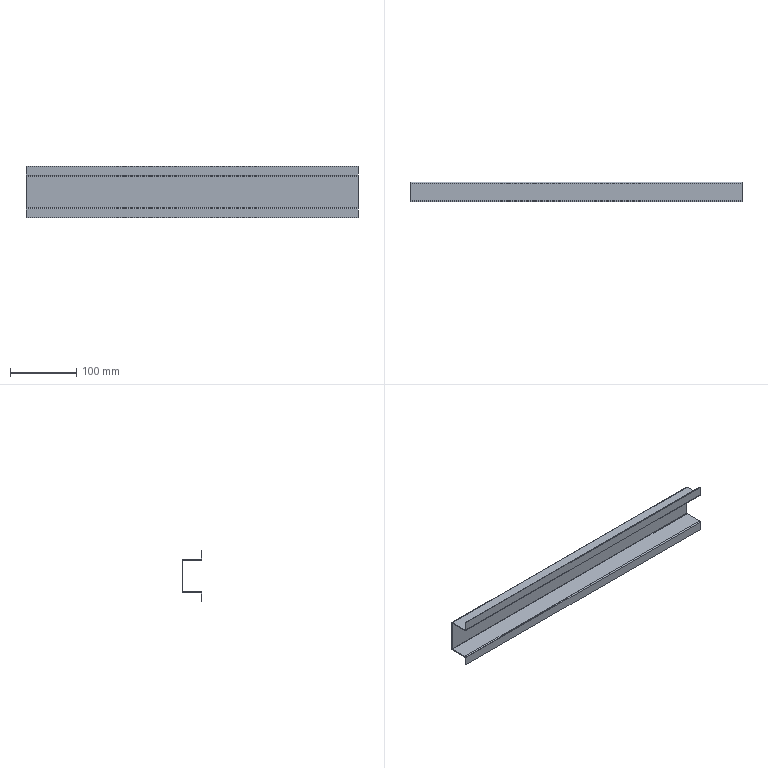Part | SolidWorks | features EdgeFlange 2, FlatPattern 1, SMBaseFlange 1, SheetMetal 1 | 1 solid | 38 faces | box 500 x 30 x 77.6 mm | volume 80038 mm3 | plane 30 | cylinder 8 | commonest cylinder face diameters 0.9 x4 3.3 x4
STEP:
#1=CARTESIAN_POINT('',(-250.,-0.45,-25.));
#2=VERTEX_POINT('',#1);
#3=CARTESIAN_POINT('',(-250.,-27.15,-25.));
#4=VERTEX_POINT('',#3);
#5=CARTESIAN_POINT('',(-250.,0.,-25.));
#6=DIRECTION('',(0.,-1.,0.));
#7=VECTOR('',#6,1000.);
#8=LINE('',#5,#7);
#9=EDGE_CURVE('',#2,#4,#8,.T.);
#10=ORIENTED_EDGE('',*,*,#9,.T.);
#11=CARTESIAN_POINT('',(-250.,-27.15,-23.8));
#12=VERTEX_POINT('',#11);
#13=CARTESIAN_POINT('',(-250.,-27.15,-25.));
#14=DIRECTION('',(0.,0.,1.));
#15=VECTOR('',#14,1000.);
#16=LINE('',#13,#15);
#17=EDGE_CURVE('',#4,#12,#16,.T.);
#18=ORIENTED_EDGE('',*,*,#17,.T.);
#19=CARTESIAN_POINT('',(-250.,-0.45,-23.8));
#20=VERTEX_POINT('',#19);
#21=CARTESIAN_POINT('',(-250.,-28.8,-23.8));
#22=DIRECTION('',(0.,-1.,0.));
#23=VECTOR('',#22,1000.);
#24=LINE('',#21,#23);
#25=EDGE_CURVE('',#20,#12,#24,.T.);
#26=ORIENTED_EDGE('',*,*,#25,.F.);
#27=CARTESIAN_POINT('',(-250.,-0.45,-25.));
#28=DIRECTION('',(0.,0.,-1.));
#29=VECTOR('',#28,1000.);
#30=LINE('',#27,#29);
#31=EDGE_CURVE('',#20,#2,#30,.T.);
#32=ORIENTED_EDGE('',*,*,#31,.T.);
#33=EDGE_LOOP('',(#10,#18,#26,#32));
#34=FACE_OUTER_BOUND('',#33,.T.);
#35=CARTESIAN_POINT('',(-250.,0.,-25.));
#36=DIRECTION('',(-1.,0.,0.));
#37=DIRECTION('',(0.,0.,1.));
#38=AXIS2_PLACEMENT_3D('',#35,#36,#37);
#39=PLANE('',#38);
#40=ADVANCED_FACE('',(#34),#39,.T.);
#41=CARTESIAN_POINT('',(250.,-27.15,-25.));
#42=VERTEX_POINT('',#41);
#43=CARTESIAN_POINT('',(-250.,-27.15,-25.));
#44=DIRECTION('',(1.,0.,0.));
#45=VECTOR('',#44,1000.);
#46=LINE('',#43,#45);
#47=EDGE_CURVE('',#4,#42,#46,.T.);
#48=ORIENTED_EDGE('',*,*,#47,.F.);
#49=ORIENTED_EDGE('',*,*,#9,.F.);
#50=CARTESIAN_POINT('',(250.,-0.45,-25.));
#51=VERTEX_POINT('',#50);
#52=CARTESIAN_POINT('',(-250.,-0.45,-25.));
#53=DIRECTION('',(-1.,0.,0.));
#54=VECTOR('',#53,1000.);
#55=LINE('',#52,#54);
#56=EDGE_CURVE('',#51,#2,#55,.T.);
#57=ORIENTED_EDGE('',*,*,#56,.F.);
#58=CARTESIAN_POINT('',(250.,-28.8,-25.));
#59=DIRECTION('',(0.,1.,0.));
#60=VECTOR('',#59,1000.);
#61=LINE('',#58,#60);
#62=EDGE_CURVE('',#42,#51,#61,.T.);
#63=ORIENTED_EDGE('',*,*,#62,.F.);
#64=EDGE_LOOP('',(#48,#49,#57,#63));
#65=FACE_OUTER_BOUND('',#64,.T.);
#66=CARTESIAN_POINT('',(-250.,-28.8,-25.));
#67=DIRECTION('',(0.,0.,1.));
#68=DIRECTION('',(0.,-1.,0.));
#69=AXIS2_PLACEMENT_3D('',#66,#67,#68);
#70=PLANE('',#69);
#71=ADVANCED_FACE('',(#65),#70,.F.);
#72=ORIENTED_EDGE('',*,*,#25,.T.);
#73=CARTESIAN_POINT('',(250.,-27.15,-23.8));
#74=VERTEX_POINT('',#73);
#75=CARTESIAN_POINT('',(-250.,-27.15,-23.8));
#76=DIRECTION('',(1.,0.,0.));
#77=VECTOR('',#76,1000.);
#78=LINE('',#75,#77);
#79=EDGE_CURVE('',#12,#74,#78,.T.);
#80=ORIENTED_EDGE('',*,*,#79,.T.);
#81=CARTESIAN_POINT('',(250.,-0.45,-23.8));
#82=VERTEX_POINT('',#81);
#83=CARTESIAN_POINT('',(250.,-28.8,-23.8));
#84=DIRECTION('',(0.,1.,0.));
#85=VECTOR('',#84,1000.);
#86=LINE('',#83,#85);
#87=EDGE_CURVE('',#74,#82,#86,.T.);
#88=ORIENTED_EDGE('',*,*,#87,.T.);
#89=CARTESIAN_POINT('',(-250.,-0.45,-23.8));
#90=DIRECTION('',(1.,0.,0.));
#91=VECTOR('',#90,1000.);
#92=LINE('',#89,#91);
#93=EDGE_CURVE('',#20,#82,#92,.T.);
#94=ORIENTED_EDGE('',*,*,#93,.F.);
#95=EDGE_LOOP('',(#72,#80,#88,#94));
#96=FACE_OUTER_BOUND('',#95,.T.);
#97=CARTESIAN_POINT('',(-250.,-28.8,-23.8));
#98=DIRECTION('',(0.,0.,1.));
#99=DIRECTION('',(0.,-1.,0.));
#100=AXIS2_PLACEMENT_3D('',#97,#98,#99);
#101=PLANE('',#100);
#102=ADVANCED_FACE('',(#96),#101,.T.);
#103=CARTESIAN_POINT('',(250.,-0.45,25.));
#104=VERTEX_POINT('',#103);
#105=CARTESIAN_POINT('',(250.,-27.15,25.));
#106=VERTEX_POINT('',#105);
#107=CARTESIAN_POINT('',(250.,-28.8,25.));
#108=DIRECTION('',(0.,-1.,0.));
#109=VECTOR('',#108,1000.);
#110=LINE('',#107,#109);
#111=EDGE_CURVE('',#104,#106,#110,.T.);
#112=ORIENTED_EDGE('',*,*,#111,.T.);
#113=CARTESIAN_POINT('',(250.,-27.15,23.8));
#114=VERTEX_POINT('',#113);
#115=CARTESIAN_POINT('',(250.,-27.15,25.));
#116=DIRECTION('',(0.,0.,-1.));
#117=VECTOR('',#116,1000.);
#118=LINE('',#115,#117);
#119=EDGE_CURVE('',#106,#114,#118,.T.);
#120=ORIENTED_EDGE('',*,*,#119,.T.);
#121=CARTESIAN_POINT('',(250.,-0.45,23.8));
#122=VERTEX_POINT('',#121);
#123=CARTESIAN_POINT('',(250.,0.,23.8));
#124=DIRECTION('',(0.,-1.,0.));
#125=VECTOR('',#124,1000.);
#126=LINE('',#123,#125);
#127=EDGE_CURVE('',#122,#114,#126,.T.);
#128=ORIENTED_EDGE('',*,*,#127,.F.);
#129=CARTESIAN_POINT('',(250.,-0.45,25.));
#130=DIRECTION('',(0.,0.,1.));
#131=VECTOR('',#130,1000.);
#132=LINE('',#129,#131);
#133=EDGE_CURVE('',#122,#104,#132,.T.);
#134=ORIENTED_EDGE('',*,*,#133,.T.);
#135=EDGE_LOOP('',(#112,#120,#128,#134));
#136=FACE_OUTER_BOUND('',#135,.T.);
#137=CARTESIAN_POINT('',(250.,-28.8,25.));
#138=DIRECTION('',(1.,0.,0.));
#139=DIRECTION('',(0.,0.,-1.));
#140=AXIS2_PLACEMENT_3D('',#137,#138,#139);
#141=PLANE('',#140);
#142=ADVANCED_FACE('',(#136),#141,.T.);
#143=CARTESIAN_POINT('',(-250.,-27.15,25.));
#144=VERTEX_POINT('',#143);
#145=CARTESIAN_POINT('',(-250.,-0.45,25.));
#146=VERTEX_POINT('',#145);
#147=CARTESIAN_POINT('',(-250.,0.,25.));
#148=DIRECTION('',(0.,1.,0.));
#149=VECTOR('',#148,1000.);
#150=LINE('',#147,#149);
#151=EDGE_CURVE('',#144,#146,#150,.T.);
#152=ORIENTED_EDGE('',*,*,#151,.F.);
#153=CARTESIAN_POINT('',(250.,-27.15,25.));
#154=DIRECTION('',(-1.,0.,0.));
#155=VECTOR('',#154,1000.);
#156=LINE('',#153,#155);
#157=EDGE_CURVE('',#106,#144,#156,.T.);
#158=ORIENTED_EDGE('',*,*,#157,.F.);
#159=ORIENTED_EDGE('',*,*,#111,.F.);
#160=CARTESIAN_POINT('',(-250.,-0.45,25.));
#161=DIRECTION('',(-1.,0.,0.));
#162=VECTOR('',#161,1000.);
#163=LINE('',#160,#162);
#164=EDGE_CURVE('',#104,#146,#163,.T.);
#165=ORIENTED_EDGE('',*,*,#164,.T.);
#166=EDGE_LOOP('',(#152,#158,#159,#165));
#167=FACE_OUTER_BOUND('',#166,.T.);
#168=CARTESIAN_POINT('',(-250.,0.,25.));
#169=DIRECTION('',(0.,0.,1.));
#170=DIRECTION('',(0.,-1.,0.));
#171=AXIS2_PLACEMENT_3D('',#168,#169,#170);
#172=PLANE('',#171);
#173=ADVANCED_FACE('',(#167),#172,.T.);
#174=CARTESIAN_POINT('',(-250.,-27.15,23.8));
#175=VERTEX_POINT('',#174);
#176=CARTESIAN_POINT('',(250.,-27.15,23.8));
#177=DIRECTION('',(-1.,0.,0.));
#178=VECTOR('',#177,1000.);
#179=LINE('',#176,#178);
#180=EDGE_CURVE('',#114,#175,#179,.T.);
#181=ORIENTED_EDGE('',*,*,#180,.T.);
#182=CARTESIAN_POINT('',(-250.,-0.45,23.8));
#183=VERTEX_POINT('',#182);
#184=CARTESIAN_POINT('',(-250.,0.,23.8));
#185=DIRECTION('',(0.,1.,0.));
#186=VECTOR('',#185,1000.);
#187=LINE('',#184,#186);
#188=EDGE_CURVE('',#175,#183,#187,.T.);
#189=ORIENTED_EDGE('',*,*,#188,.T.);
#190=CARTESIAN_POINT('',(250.,-0.45,23.8));
#191=DIRECTION('',(-1.,0.,0.));
#192=VECTOR('',#191,1000.);
#193=LINE('',#190,#192);
#194=EDGE_CURVE('',#122,#183,#193,.T.);
#195=ORIENTED_EDGE('',*,*,#194,.F.);
#196=ORIENTED_EDGE('',*,*,#127,.T.);
#197=EDGE_LOOP('',(#181,#189,#195,#196));
#198=FACE_OUTER_BOUND('',#197,.T.);
#199=CARTESIAN_POINT('',(-250.,0.,23.8));
#200=DIRECTION('',(0.,0.,1.));
#201=DIRECTION('',(0.,-1.,0.));
#202=AXIS2_PLACEMENT_3D('',#199,#200,#201);
#203=PLANE('',#202);
#204=ADVANCED_FACE('',(#198),#203,.F.);
#205=CARTESIAN_POINT('',(-250.,0.,-23.35));
#206=VERTEX_POINT('',#205);
#207=CARTESIAN_POINT('',(-250.,1.2,-23.35));
#208=VERTEX_POINT('',#207);
#209=CARTESIAN_POINT('',(-250.,0.,-23.35));
#210=DIRECTION('',(0.,1.,0.));
#211=VECTOR('',#210,1000.);
#212=LINE('',#209,#211);
#213=EDGE_CURVE('',#206,#208,#212,.T.);
#214=ORIENTED_EDGE('',*,*,#213,.F.);
#215=CARTESIAN_POINT('',(-250.,0.,23.35));
#216=VERTEX_POINT('',#215);
#217=CARTESIAN_POINT('',(-250.,0.,-25.));
#218=DIRECTION('',(0.,0.,1.));
#219=VECTOR('',#218,1000.);
#220=LINE('',#217,#219);
#221=EDGE_CURVE('',#206,#216,#220,.T.);
#222=ORIENTED_EDGE('',*,*,#221,.T.);
#223=CARTESIAN_POINT('',(-250.,1.2,23.35));
#224=VERTEX_POINT('',#223);
#225=CARTESIAN_POINT('',(-250.,0.,23.35));
#226=DIRECTION('',(0.,1.,0.));
#227=VECTOR('',#226,1000.);
#228=LINE('',#225,#227);
#229=EDGE_CURVE('',#216,#224,#228,.T.);
#230=ORIENTED_EDGE('',*,*,#229,.T.);
#231=CARTESIAN_POINT('',(-250.,1.2,-25.));
#232=DIRECTION('',(0.,0.,1.));
#233=VECTOR('',#232,1000.);
#234=LINE('',#231,#233);
#235=EDGE_CURVE('',#208,#224,#234,.T.);
#236=ORIENTED_EDGE('',*,*,#235,.F.);
#237=EDGE_LOOP('',(#214,#222,#230,#236));
#238=FACE_OUTER_BOUND('',#237,.T.);
#239=CARTESIAN_POINT('',(-250.,1.2,-25.));
#240=DIRECTION('',(1.,0.,0.));
#241=DIRECTION('',(0.,0.,-1.));
#242=AXIS2_PLACEMENT_3D('',#239,#240,#241);
#243=PLANE('',#242);
#244=ADVANCED_FACE('',(#238),#243,.F.);
#245=CARTESIAN_POINT('',(250.,0.,-23.35));
#246=VERTEX_POINT('',#245);
#247=CARTESIAN_POINT('',(250.,1.2,-23.35));
#248=VERTEX_POINT('',#247);
#249=CARTESIAN_POINT('',(250.,0.,-23.35));
#250=DIRECTION('',(0.,1.,0.));
#251=VECTOR('',#250,1000.);
#252=LINE('',#249,#251);
#253=EDGE_CURVE('',#246,#248,#252,.T.);
#254=ORIENTED_EDGE('',*,*,#253,.T.);
#255=CARTESIAN_POINT('',(250.,1.2,23.35));
#256=VERTEX_POINT('',#255);
#257=CARTESIAN_POINT('',(250.,1.2,-25.));
#258=DIRECTION('',(0.,0.,-1.));
#259=VECTOR('',#258,1000.);
#260=LINE('',#257,#259);
#261=EDGE_CURVE('',#256,#248,#260,.T.);
#262=ORIENTED_EDGE('',*,*,#261,.F.);
#263=CARTESIAN_POINT('',(250.,0.,23.35));
#264=VERTEX_POINT('',#263);
#265=CARTESIAN_POINT('',(250.,0.,23.35));
#266=DIRECTION('',(0.,1.,0.));
#267=VECTOR('',#266,1000.);
#268=LINE('',#265,#267);
#269=EDGE_CURVE('',#264,#256,#268,.T.);
#270=ORIENTED_EDGE('',*,*,#269,.F.);
#271=CARTESIAN_POINT('',(250.,0.,-25.));
#272=DIRECTION('',(0.,0.,-1.));
#273=VECTOR('',#272,1000.);
#274=LINE('',#271,#273);
#275=EDGE_CURVE('',#264,#246,#274,.T.);
#276=ORIENTED_EDGE('',*,*,#275,.T.);
#277=EDGE_LOOP('',(#254,#262,#270,#276));
#278=FACE_OUTER_BOUND('',#277,.T.);
#279=CARTESIAN_POINT('',(250.,1.2,-25.));
#280=DIRECTION('',(-1.,0.,0.));
#281=DIRECTION('',(0.,0.,1.));
#282=AXIS2_PLACEMENT_3D('',#279,#280,#281);
#283=PLANE('',#282);
#284=ADVANCED_FACE('',(#278),#283,.F.);
#285=ORIENTED_EDGE('',*,*,#261,.T.);
#286=CARTESIAN_POINT('',(250.,1.2,-23.35));
#287=DIRECTION('',(-1.,0.,0.));
#288=VECTOR('',#287,1000.);
#289=LINE('',#286,#288);
#290=EDGE_CURVE('',#248,#208,#289,.T.);
#291=ORIENTED_EDGE('',*,*,#290,.T.);
#292=ORIENTED_EDGE('',*,*,#235,.T.);
#293=CARTESIAN_POINT('',(-250.,1.2,23.35));
#294=DIRECTION('',(1.,0.,0.));
#295=VECTOR('',#294,1000.);
#296=LINE('',#293,#295);
#297=EDGE_CURVE('',#224,#256,#296,.T.);
#298=ORIENTED_EDGE('',*,*,#297,.T.);
#299=EDGE_LOOP('',(#285,#291,#292,#298));
#300=FACE_OUTER_BOUND('',#299,.T.);
#301=CARTESIAN_POINT('',(-250.,1.2,25.));
#302=DIRECTION('',(0.,1.,0.));
#303=DIRECTION('',(0.,0.,1.));
#304=AXIS2_PLACEMENT_3D('',#301,#302,#303);
#305=PLANE('',#304);
#306=ADVANCED_FACE('',(#300),#305,.T.);
#307=CARTESIAN_POINT('',(250.,0.,-23.35));
#308=DIRECTION('',(-1.,0.,0.));
#309=VECTOR('',#308,1000.);
#310=LINE('',#307,#309);
#311=EDGE_CURVE('',#246,#206,#310,.T.);
#312=ORIENTED_EDGE('',*,*,#311,.F.);
#313=ORIENTED_EDGE('',*,*,#275,.F.);
#314=CARTESIAN_POINT('',(-250.,0.,23.35));
#315=DIRECTION('',(1.,0.,0.));
#316=VECTOR('',#315,1000.);
#317=LINE('',#314,#316);
#318=EDGE_CURVE('',#216,#264,#317,.T.);
#319=ORIENTED_EDGE('',*,*,#318,.F.);
#320=ORIENTED_EDGE('',*,*,#221,.F.);
#321=EDGE_LOOP('',(#312,#313,#319,#320));
#322=FACE_OUTER_BOUND('',#321,.T.);
#323=CARTESIAN_POINT('',(-250.,0.,25.));
#324=DIRECTION('',(0.,1.,0.));
#325=DIRECTION('',(0.,0.,1.));
#326=AXIS2_PLACEMENT_3D('',#323,#324,#325);
#327=PLANE('',#326);
#328=ADVANCED_FACE('',(#322),#327,.F.);
#329=ORIENTED_EDGE('',*,*,#133,.F.);
#330=CARTESIAN_POINT('',(250.,-0.45,23.35));
#331=DIRECTION('',(1.,0.,0.));
#332=DIRECTION('',(0.,0.,1.));
#333=AXIS2_PLACEMENT_3D('',#330,#331,#332);
#334=CIRCLE('',#333,0.45);
#335=EDGE_CURVE('',#264,#122,#334,.T.);
#336=ORIENTED_EDGE('',*,*,#335,.F.);
#337=ORIENTED_EDGE('',*,*,#269,.T.);
#338=CARTESIAN_POINT('',(250.,-0.45,23.35));
#339=DIRECTION('',(1.,0.,0.));
#340=DIRECTION('',(0.,0.,1.));
#341=AXIS2_PLACEMENT_3D('',#338,#339,#340);
#342=CIRCLE('',#341,1.65);
#343=EDGE_CURVE('',#256,#104,#342,.T.);
#344=ORIENTED_EDGE('',*,*,#343,.T.);
#345=EDGE_LOOP('',(#329,#336,#337,#344));
#346=FACE_OUTER_BOUND('',#345,.T.);
#347=CARTESIAN_POINT('',(250.,-0.45,23.35));
#348=DIRECTION('',(1.,0.,0.));
#349=DIRECTION('',(0.,0.,-1.));
#350=AXIS2_PLACEMENT_3D('',#347,#348,#349);
#351=PLANE('',#350);
#352=ADVANCED_FACE('',(#346),#351,.T.);
#353=ORIENTED_EDGE('',*,*,#297,.F.);
#354=CARTESIAN_POINT('',(-250.,-0.45,23.35));
#355=DIRECTION('',(-1.,0.,0.));
#356=DIRECTION('',(0.,0.,1.));
#357=AXIS2_PLACEMENT_3D('',#354,#355,#356);
#358=CIRCLE('',#357,1.65);
#359=EDGE_CURVE('',#146,#224,#358,.T.);
#360=ORIENTED_EDGE('',*,*,#359,.F.);
#361=ORIENTED_EDGE('',*,*,#164,.F.);
#362=ORIENTED_EDGE('',*,*,#343,.F.);
#363=EDGE_LOOP('',(#353,#360,#361,#362));
#364=FACE_OUTER_BOUND('',#363,.T.);
#365=CARTESIAN_POINT('',(-250.,-0.45,23.35));
#366=DIRECTION('',(-1.,0.,0.));
#367=DIRECTION('',(0.,0.,1.));
#368=AXIS2_PLACEMENT_3D('',#365,#366,#367);
#369=CYLINDRICAL_SURFACE('',#368,1.65);
#370=ADVANCED_FACE('',(#364),#369,.T.);
#371=CARTESIAN_POINT('',(-250.,-0.45,23.35));
#372=DIRECTION('',(-1.,0.,0.));
#373=DIRECTION('',(0.,0.,1.));
#374=AXIS2_PLACEMENT_3D('',#371,#372,#373);
#375=CIRCLE('',#374,0.45);
#376=EDGE_CURVE('',#183,#216,#375,.T.);
#377=ORIENTED_EDGE('',*,*,#376,.F.);
#378=CARTESIAN_POINT('',(-250.,-0.45,23.8));
#379=DIRECTION('',(0.,0.,1.));
#380=VECTOR('',#379,1000.);
#381=LINE('',#378,#380);
#382=EDGE_CURVE('',#183,#146,#381,.T.);
#383=ORIENTED_EDGE('',*,*,#382,.T.);
#384=ORIENTED_EDGE('',*,*,#359,.T.);
#385=ORIENTED_EDGE('',*,*,#229,.F.);
#386=EDGE_LOOP('',(#377,#383,#384,#385));
#387=FACE_OUTER_BOUND('',#386,.T.);
#388=CARTESIAN_POINT('',(-250.,-0.45,23.35));
#389=DIRECTION('',(1.,0.,0.));
#390=DIRECTION('',(0.,0.,-1.));
#391=AXIS2_PLACEMENT_3D('',#388,#389,#390);
#392=PLANE('',#391);
#393=ADVANCED_FACE('',(#387),#392,.F.);
#394=ORIENTED_EDGE('',*,*,#318,.T.);
#395=ORIENTED_EDGE('',*,*,#335,.T.);
#396=ORIENTED_EDGE('',*,*,#194,.T.);
#397=ORIENTED_EDGE('',*,*,#376,.T.);
#398=EDGE_LOOP('',(#394,#395,#396,#397));
#399=FACE_OUTER_BOUND('',#398,.T.);
#400=CARTESIAN_POINT('',(-250.,-0.45,23.35));
#401=DIRECTION('',(-1.,0.,0.));
#402=DIRECTION('',(0.,0.,1.));
#403=AXIS2_PLACEMENT_3D('',#400,#401,#402);
#404=CYLINDRICAL_SURFACE('',#403,0.45);
#405=ADVANCED_FACE('',(#399),#404,.F.);
#406=CARTESIAN_POINT('',(-250.,-27.15,25.));
#407=DIRECTION('',(0.,0.,-1.));
#408=VECTOR('',#407,1000.);
#409=LINE('',#406,#408);
#410=EDGE_CURVE('',#144,#175,#409,.T.);
#411=ORIENTED_EDGE('',*,*,#410,.F.);
#412=ORIENTED_EDGE('',*,*,#151,.T.);
#413=ORIENTED_EDGE('',*,*,#382,.F.);
#414=ORIENTED_EDGE('',*,*,#188,.F.);
#415=EDGE_LOOP('',(#411,#412,#413,#414));
#416=FACE_OUTER_BOUND('',#415,.T.);
#417=CARTESIAN_POINT('',(-250.,0.,25.));
#418=DIRECTION('',(-1.,0.,0.));
#419=DIRECTION('',(0.,0.,1.));
#420=AXIS2_PLACEMENT_3D('',#417,#418,#419);
#421=PLANE('',#420);
#422=ADVANCED_FACE('',(#416),#421,.T.);
#423=ORIENTED_EDGE('',*,*,#31,.F.);
#424=CARTESIAN_POINT('',(-250.,-0.45,-23.35));
#425=DIRECTION('',(-1.,0.,0.));
#426=DIRECTION('',(0.,0.,-1.));
#427=AXIS2_PLACEMENT_3D('',#424,#425,#426);
#428=CIRCLE('',#427,0.45);
#429=EDGE_CURVE('',#206,#20,#428,.T.);
#430=ORIENTED_EDGE('',*,*,#429,.F.);
#431=ORIENTED_EDGE('',*,*,#213,.T.);
#432=CARTESIAN_POINT('',(-250.,-0.45,-23.35));
#433=DIRECTION('',(-1.,0.,0.));
#434=DIRECTION('',(0.,0.,-1.));
#435=AXIS2_PLACEMENT_3D('',#432,#433,#434);
#436=CIRCLE('',#435,1.65);
#437=EDGE_CURVE('',#208,#2,#436,.T.);
#438=ORIENTED_EDGE('',*,*,#437,.T.);
#439=EDGE_LOOP('',(#423,#430,#431,#438));
#440=FACE_OUTER_BOUND('',#439,.T.);
#441=CARTESIAN_POINT('',(-250.,-0.45,-23.35));
#442=DIRECTION('',(-1.,0.,0.));
#443=DIRECTION('',(0.,0.,1.));
#444=AXIS2_PLACEMENT_3D('',#441,#442,#443);
#445=PLANE('',#444);
#446=ADVANCED_FACE('',(#440),#445,.T.);
#447=ORIENTED_EDGE('',*,*,#290,.F.);
#448=CARTESIAN_POINT('',(250.,-0.45,-23.35));
#449=DIRECTION('',(1.,0.,0.));
#450=DIRECTION('',(0.,0.,-1.));
#451=AXIS2_PLACEMENT_3D('',#448,#449,#450);
#452=CIRCLE('',#451,1.65);
#453=EDGE_CURVE('',#51,#248,#452,.T.);
#454=ORIENTED_EDGE('',*,*,#453,.F.);
#455=ORIENTED_EDGE('',*,*,#56,.T.);
#456=ORIENTED_EDGE('',*,*,#437,.F.);
#457=EDGE_LOOP('',(#447,#454,#455,#456));
#458=FACE_OUTER_BOUND('',#457,.T.);
#459=CARTESIAN_POINT('',(250.,-0.45,-23.35));
#460=DIRECTION('',(1.,0.,0.));
#461=DIRECTION('',(0.,0.,-1.));
#462=AXIS2_PLACEMENT_3D('',#459,#460,#461);
#463=CYLINDRICAL_SURFACE('',#462,1.65);
#464=ADVANCED_FACE('',(#458),#463,.T.);
#465=CARTESIAN_POINT('',(250.,-0.45,-23.35));
#466=DIRECTION('',(1.,0.,0.));
#467=DIRECTION('',(0.,0.,-1.));
#468=AXIS2_PLACEMENT_3D('',#465,#466,#467);
#469=CIRCLE('',#468,0.45);
#470=EDGE_CURVE('',#82,#246,#469,.T.);
#471=ORIENTED_EDGE('',*,*,#470,.F.);
#472=CARTESIAN_POINT('',(250.,-0.45,-23.8));
#473=DIRECTION('',(0.,0.,-1.));
#474=VECTOR('',#473,1000.);
#475=LINE('',#472,#474);
#476=EDGE_CURVE('',#82,#51,#475,.T.);
#477=ORIENTED_EDGE('',*,*,#476,.T.);
#478=ORIENTED_EDGE('',*,*,#453,.T.);
#479=ORIENTED_EDGE('',*,*,#253,.F.);
#480=EDGE_LOOP('',(#471,#477,#478,#479));
#481=FACE_OUTER_BOUND('',#480,.T.);
#482=CARTESIAN_POINT('',(250.,-0.45,-23.35));
#483=DIRECTION('',(-1.,0.,0.));
#484=DIRECTION('',(0.,0.,1.));
#485=AXIS2_PLACEMENT_3D('',#482,#483,#484);
#486=PLANE('',#485);
#487=ADVANCED_FACE('',(#481),#486,.F.);
#488=ORIENTED_EDGE('',*,*,#311,.T.);
#489=ORIENTED_EDGE('',*,*,#429,.T.);
#490=ORIENTED_EDGE('',*,*,#93,.T.);
#491=ORIENTED_EDGE('',*,*,#470,.T.);
#492=EDGE_LOOP('',(#488,#489,#490,#491));
#493=FACE_OUTER_BOUND('',#492,.T.);
#494=CARTESIAN_POINT('',(250.,-0.45,-23.35));
#495=DIRECTION('',(1.,0.,0.));
#496=DIRECTION('',(0.,0.,-1.));
#497=AXIS2_PLACEMENT_3D('',#494,#495,#496);
#498=CYLINDRICAL_SURFACE('',#497,0.45);
#499=ADVANCED_FACE('',(#493),#498,.F.);
#500=CARTESIAN_POINT('',(250.,-27.15,-25.));
#501=DIRECTION('',(0.,0.,1.));
#502=VECTOR('',#501,1000.);
#503=LINE('',#500,#502);
#504=EDGE_CURVE('',#42,#74,#503,.T.);
#505=ORIENTED_EDGE('',*,*,#504,.F.);
#506=ORIENTED_EDGE('',*,*,#62,.T.);
#507=ORIENTED_EDGE('',*,*,#476,.F.);
#508=ORIENTED_EDGE('',*,*,#87,.F.);
#509=EDGE_LOOP('',(#505,#506,#507,#508));
#510=FACE_OUTER_BOUND('',#509,.T.);
#511=CARTESIAN_POINT('',(250.,-28.8,-25.));
#512=DIRECTION('',(1.,0.,0.));
#513=DIRECTION('',(0.,0.,-1.));
#514=AXIS2_PLACEMENT_3D('',#511,#512,#513);
#515=PLANE('',#514);
#516=ADVANCED_FACE('',(#510),#515,.T.);
#517=CARTESIAN_POINT('',(-250.,-27.6,25.45));
#518=VERTEX_POINT('',#517);
#519=CARTESIAN_POINT('',(-250.,-28.8,25.45));
#520=VERTEX_POINT('',#519);
#521=CARTESIAN_POINT('',(-250.,-28.8,25.45));
#522=DIRECTION('',(0.,-1.,0.));
#523=VECTOR('',#522,1000.);
#524=LINE('',#521,#523);
#525=EDGE_CURVE('',#518,#520,#524,.T.);
#526=ORIENTED_EDGE('',*,*,#525,.F.);
#527=CARTESIAN_POINT('',(-250.,-27.15,25.45));
#528=DIRECTION('',(-1.,0.,0.));
#529=DIRECTION('',(0.,0.,-1.));
#530=AXIS2_PLACEMENT_3D('',#527,#528,#529);
#531=CIRCLE('',#530,0.45);
#532=EDGE_CURVE('',#144,#518,#531,.T.);
#533=ORIENTED_EDGE('',*,*,#532,.F.);
#534=ORIENTED_EDGE('',*,*,#410,.T.);
#535=CARTESIAN_POINT('',(-250.,-27.15,25.45));
#536=DIRECTION('',(-1.,0.,0.));
#537=DIRECTION('',(0.,0.,-1.));
#538=AXIS2_PLACEMENT_3D('',#535,#536,#537);
#539=CIRCLE('',#538,1.65);
#540=EDGE_CURVE('',#175,#520,#539,.T.);
#541=ORIENTED_EDGE('',*,*,#540,.T.);
#542=EDGE_LOOP('',(#526,#533,#534,#541));
#543=FACE_OUTER_BOUND('',#542,.T.);
#544=CARTESIAN_POINT('',(-250.,-27.15,25.45));
#545=DIRECTION('',(-1.,0.,0.));
#546=DIRECTION('',(0.,0.,1.));
#547=AXIS2_PLACEMENT_3D('',#544,#545,#546);
#548=PLANE('',#547);
#549=ADVANCED_FACE('',(#543),#548,.T.);
#550=ORIENTED_EDGE('',*,*,#180,.F.);
#551=CARTESIAN_POINT('',(250.,-28.8,25.45));
#552=VERTEX_POINT('',#551);
#553=CARTESIAN_POINT('',(250.,-27.15,25.45));
#554=DIRECTION('',(1.,0.,0.));
#555=DIRECTION('',(0.,0.,-1.));
#556=AXIS2_PLACEMENT_3D('',#553,#554,#555);
#557=CIRCLE('',#556,1.65);
#558=EDGE_CURVE('',#552,#114,#557,.T.);
#559=ORIENTED_EDGE('',*,*,#558,.F.);
#560=CARTESIAN_POINT('',(-250.,-28.8,25.45));
#561=DIRECTION('',(-1.,0.,0.));
#562=VECTOR('',#561,1000.);
#563=LINE('',#560,#562);
#564=EDGE_CURVE('',#552,#520,#563,.T.);
#565=ORIENTED_EDGE('',*,*,#564,.T.);
#566=ORIENTED_EDGE('',*,*,#540,.F.);
#567=EDGE_LOOP('',(#550,#559,#565,#566));
#568=FACE_OUTER_BOUND('',#567,.T.);
#569=CARTESIAN_POINT('',(250.,-27.15,25.45));
#570=DIRECTION('',(1.,0.,0.));
#571=DIRECTION('',(0.,-1.,0.));
#572=AXIS2_PLACEMENT_3D('',#569,#570,#571);
#573=CYLINDRICAL_SURFACE('',#572,1.65);
#574=ADVANCED_FACE('',(#568),#573,.T.);
#575=CARTESIAN_POINT('',(250.,-27.6,25.45));
#576=VERTEX_POINT('',#575);
#577=CARTESIAN_POINT('',(250.,-27.15,25.45));
#578=DIRECTION('',(1.,0.,0.));
#579=DIRECTION('',(0.,0.,-1.));
#580=AXIS2_PLACEMENT_3D('',#577,#578,#579);
#581=CIRCLE('',#580,0.45);
#582=EDGE_CURVE('',#576,#106,#581,.T.);
#583=ORIENTED_EDGE('',*,*,#582,.F.);
#584=CARTESIAN_POINT('',(250.,-27.6,25.45));
#585=DIRECTION('',(0.,-1.,0.));
#586=VECTOR('',#585,1000.);
#587=LINE('',#584,#586);
#588=EDGE_CURVE('',#576,#552,#587,.T.);
#589=ORIENTED_EDGE('',*,*,#588,.T.);
#590=ORIENTED_EDGE('',*,*,#558,.T.);
#591=ORIENTED_EDGE('',*,*,#119,.F.);
#592=EDGE_LOOP('',(#583,#589,#590,#591));
#593=FACE_OUTER_BOUND('',#592,.T.);
#594=CARTESIAN_POINT('',(250.,-27.15,25.45));
#595=DIRECTION('',(-1.,0.,0.));
#596=DIRECTION('',(0.,0.,1.));
#597=AXIS2_PLACEMENT_3D('',#594,#595,#596);
#598=PLANE('',#597);
#599=ADVANCED_FACE('',(#593),#598,.F.);
#600=ORIENTED_EDGE('',*,*,#157,.T.);
#601=ORIENTED_EDGE('',*,*,#532,.T.);
#602=CARTESIAN_POINT('',(-250.,-27.6,25.45));
#603=DIRECTION('',(1.,0.,0.));
#604=VECTOR('',#603,1000.);
#605=LINE('',#602,#604);
#606=EDGE_CURVE('',#518,#576,#605,.T.);
#607=ORIENTED_EDGE('',*,*,#606,.T.);
#608=ORIENTED_EDGE('',*,*,#582,.T.);
#609=EDGE_LOOP('',(#600,#601,#607,#608));
#610=FACE_OUTER_BOUND('',#609,.T.);
#611=CARTESIAN_POINT('',(250.,-27.15,25.45));
#612=DIRECTION('',(1.,0.,0.));
#613=DIRECTION('',(0.,-1.,0.));
#614=AXIS2_PLACEMENT_3D('',#611,#612,#613);
#615=CYLINDRICAL_SURFACE('',#614,0.45);
#616=ADVANCED_FACE('',(#610),#615,.F.);
#617=ORIENTED_EDGE('',*,*,#588,.F.);
#618=CARTESIAN_POINT('',(250.,-27.6,38.8));
#619=VERTEX_POINT('',#618);
#620=CARTESIAN_POINT('',(250.,-27.6,38.8));
#621=DIRECTION('',(0.,0.,1.));
#622=VECTOR('',#621,1000.);
#623=LINE('',#620,#622);
#624=EDGE_CURVE('',#576,#619,#623,.T.);
#625=ORIENTED_EDGE('',*,*,#624,.T.);
#626=CARTESIAN_POINT('',(250.,-28.8,38.8));
#627=VERTEX_POINT('',#626);
#628=CARTESIAN_POINT('',(250.,-28.8,38.8));
#629=DIRECTION('',(0.,1.,0.));
#630=VECTOR('',#629,1000.);
#631=LINE('',#628,#630);
#632=EDGE_CURVE('',#627,#619,#631,.T.);
#633=ORIENTED_EDGE('',*,*,#632,.F.);
#634=CARTESIAN_POINT('',(250.,-28.8,25.));
#635=DIRECTION('',(0.,0.,1.));
#636=VECTOR('',#635,1000.);
#637=LINE('',#634,#636);
#638=EDGE_CURVE('',#552,#627,#637,.T.);
#639=ORIENTED_EDGE('',*,*,#638,.F.);
#640=EDGE_LOOP('',(#617,#625,#633,#639));
#641=FACE_OUTER_BOUND('',#640,.T.);
#642=CARTESIAN_POINT('',(250.,-28.8,38.8));
#643=DIRECTION('',(-1.,0.,0.));
#644=DIRECTION('',(0.,0.,1.));
#645=AXIS2_PLACEMENT_3D('',#642,#643,#644);
#646=PLANE('',#645);
#647=ADVANCED_FACE('',(#641),#646,.F.);
#648=ORIENTED_EDGE('',*,*,#525,.T.);
#649=CARTESIAN_POINT('',(-250.,-28.8,38.8));
#650=VERTEX_POINT('',#649);
#651=CARTESIAN_POINT('',(-250.,-28.8,25.));
#652=DIRECTION('',(0.,0.,-1.));
#653=VECTOR('',#652,1000.);
#654=LINE('',#651,#653);
#655=EDGE_CURVE('',#650,#520,#654,.T.);
#656=ORIENTED_EDGE('',*,*,#655,.F.);
#657=CARTESIAN_POINT('',(-250.,-27.6,38.8));
#658=VERTEX_POINT('',#657);
#659=CARTESIAN_POINT('',(-250.,-28.8,38.8));
#660=DIRECTION('',(0.,1.,0.));
#661=VECTOR('',#660,1000.);
#662=LINE('',#659,#661);
#663=EDGE_CURVE('',#650,#658,#662,.T.);
#664=ORIENTED_EDGE('',*,*,#663,.T.);
#665=CARTESIAN_POINT('',(-250.,-27.6,25.));
#666=DIRECTION('',(0.,0.,-1.));
#667=VECTOR('',#666,1000.);
#668=LINE('',#665,#667);
#669=EDGE_CURVE('',#658,#518,#668,.T.);
#670=ORIENTED_EDGE('',*,*,#669,.T.);
#671=EDGE_LOOP('',(#648,#656,#664,#670));
#672=FACE_OUTER_BOUND('',#671,.T.);
#673=CARTESIAN_POINT('',(-250.,-28.8,25.));
#674=DIRECTION('',(1.,0.,0.));
#675=DIRECTION('',(0.,0.,-1.));
#676=AXIS2_PLACEMENT_3D('',#673,#674,#675);
#677=PLANE('',#676);
#678=ADVANCED_FACE('',(#672),#677,.F.);
#679=ORIENTED_EDGE('',*,*,#564,.F.);
#680=ORIENTED_EDGE('',*,*,#638,.T.);
#681=CARTESIAN_POINT('',(250.,-28.8,38.8));
#682=DIRECTION('',(-1.,0.,0.));
#683=VECTOR('',#682,1000.);
#684=LINE('',#681,#683);
#685=EDGE_CURVE('',#627,#650,#684,.T.);
#686=ORIENTED_EDGE('',*,*,#685,.T.);
#687=ORIENTED_EDGE('',*,*,#655,.T.);
#688=EDGE_LOOP('',(#679,#680,#686,#687));
#689=FACE_OUTER_BOUND('',#688,.T.);
#690=CARTESIAN_POINT('',(250.,-28.8,25.));
#691=DIRECTION('',(0.,1.,0.));
#692=DIRECTION('',(0.,0.,1.));
#693=AXIS2_PLACEMENT_3D('',#690,#691,#692);
#694=PLANE('',#693);
#695=ADVANCED_FACE('',(#689),#694,.F.);
#696=ORIENTED_EDGE('',*,*,#624,.F.);
#697=ORIENTED_EDGE('',*,*,#606,.F.);
#698=ORIENTED_EDGE('',*,*,#669,.F.);
#699=CARTESIAN_POINT('',(-250.,-27.6,38.8));
#700=DIRECTION('',(-1.,0.,0.));
#701=VECTOR('',#700,1000.);
#702=LINE('',#699,#701);
#703=EDGE_CURVE('',#619,#658,#702,.T.);
#704=ORIENTED_EDGE('',*,*,#703,.F.);
#705=EDGE_LOOP('',(#696,#697,#698,#704));
#706=FACE_OUTER_BOUND('',#705,.T.);
#707=CARTESIAN_POINT('',(250.,-27.6,25.));
#708=DIRECTION('',(0.,1.,0.));
#709=DIRECTION('',(0.,0.,1.));
#710=AXIS2_PLACEMENT_3D('',#707,#708,#709);
#711=PLANE('',#710);
#712=ADVANCED_FACE('',(#706),#711,.T.);
#713=ORIENTED_EDGE('',*,*,#703,.T.);
#714=ORIENTED_EDGE('',*,*,#663,.F.);
#715=ORIENTED_EDGE('',*,*,#685,.F.);
#716=ORIENTED_EDGE('',*,*,#632,.T.);
#717=EDGE_LOOP('',(#713,#714,#715,#716));
#718=FACE_OUTER_BOUND('',#717,.T.);
#719=CARTESIAN_POINT('',(-250.,-28.8,38.8));
#720=DIRECTION('',(0.,0.,-1.));
#721=DIRECTION('',(0.,1.,0.));
#722=AXIS2_PLACEMENT_3D('',#719,#720,#721);
#723=PLANE('',#722);
#724=ADVANCED_FACE('',(#718),#723,.F.);
#725=CARTESIAN_POINT('',(250.,-27.6,-25.45));
#726=VERTEX_POINT('',#725);
#727=CARTESIAN_POINT('',(250.,-28.8,-25.45));
#728=VERTEX_POINT('',#727);
#729=CARTESIAN_POINT('',(250.,-28.8,-25.45));
#730=DIRECTION('',(0.,-1.,0.));
#731=VECTOR('',#730,1000.);
#732=LINE('',#729,#731);
#733=EDGE_CURVE('',#726,#728,#732,.T.);
#734=ORIENTED_EDGE('',*,*,#733,.F.);
#735=CARTESIAN_POINT('',(250.,-27.15,-25.45));
#736=DIRECTION('',(1.,0.,0.));
#737=DIRECTION('',(0.,0.,1.));
#738=AXIS2_PLACEMENT_3D('',#735,#736,#737);
#739=CIRCLE('',#738,0.45);
#740=EDGE_CURVE('',#42,#726,#739,.T.);
#741=ORIENTED_EDGE('',*,*,#740,.F.);
#742=ORIENTED_EDGE('',*,*,#504,.T.);
#743=CARTESIAN_POINT('',(250.,-27.15,-25.45));
#744=DIRECTION('',(1.,0.,0.));
#745=DIRECTION('',(0.,0.,1.));
#746=AXIS2_PLACEMENT_3D('',#743,#744,#745);
#747=CIRCLE('',#746,1.65);
#748=EDGE_CURVE('',#74,#728,#747,.T.);
#749=ORIENTED_EDGE('',*,*,#748,.T.);
#750=EDGE_LOOP('',(#734,#741,#742,#749));
#751=FACE_OUTER_BOUND('',#750,.T.);
#752=CARTESIAN_POINT('',(250.,-27.15,-25.45));
#753=DIRECTION('',(1.,0.,0.));
#754=DIRECTION('',(0.,0.,-1.));
#755=AXIS2_PLACEMENT_3D('',#752,#753,#754);
#756=PLANE('',#755);
#757=ADVANCED_FACE('',(#751),#756,.T.);
#758=ORIENTED_EDGE('',*,*,#79,.F.);
#759=CARTESIAN_POINT('',(-250.,-28.8,-25.45));
#760=VERTEX_POINT('',#759);
#761=CARTESIAN_POINT('',(-250.,-27.15,-25.45));
#762=DIRECTION('',(-1.,0.,0.));
#763=DIRECTION('',(0.,0.,1.));
#764=AXIS2_PLACEMENT_3D('',#761,#762,#763);
#765=CIRCLE('',#764,1.65);
#766=EDGE_CURVE('',#760,#12,#765,.T.);
#767=ORIENTED_EDGE('',*,*,#766,.F.);
#768=CARTESIAN_POINT('',(250.,-28.8,-25.45));
#769=DIRECTION('',(1.,0.,0.));
#770=VECTOR('',#769,1000.);
#771=LINE('',#768,#770);
#772=EDGE_CURVE('',#760,#728,#771,.T.);
#773=ORIENTED_EDGE('',*,*,#772,.T.);
#774=ORIENTED_EDGE('',*,*,#748,.F.);
#775=EDGE_LOOP('',(#758,#767,#773,#774));
#776=FACE_OUTER_BOUND('',#775,.T.);
#777=CARTESIAN_POINT('',(-250.,-27.15,-25.45));
#778=DIRECTION('',(-1.,0.,0.));
#779=DIRECTION('',(0.,-1.,0.));
#780=AXIS2_PLACEMENT_3D('',#777,#778,#779);
#781=CYLINDRICAL_SURFACE('',#780,1.65);
#782=ADVANCED_FACE('',(#776),#781,.T.);
#783=CARTESIAN_POINT('',(-250.,-27.6,-25.45));
#784=VERTEX_POINT('',#783);
#785=CARTESIAN_POINT('',(-250.,-27.15,-25.45));
#786=DIRECTION('',(-1.,0.,0.));
#787=DIRECTION('',(0.,0.,1.));
#788=AXIS2_PLACEMENT_3D('',#785,#786,#787);
#789=CIRCLE('',#788,0.45);
#790=EDGE_CURVE('',#784,#4,#789,.T.);
#791=ORIENTED_EDGE('',*,*,#790,.F.);
#792=CARTESIAN_POINT('',(-250.,-27.6,-25.45));
#793=DIRECTION('',(0.,-1.,0.));
#794=VECTOR('',#793,1000.);
#795=LINE('',#792,#794);
#796=EDGE_CURVE('',#784,#760,#795,.T.);
#797=ORIENTED_EDGE('',*,*,#796,.T.);
#798=ORIENTED_EDGE('',*,*,#766,.T.);
#799=ORIENTED_EDGE('',*,*,#17,.F.);
#800=EDGE_LOOP('',(#791,#797,#798,#799));
#801=FACE_OUTER_BOUND('',#800,.T.);
#802=CARTESIAN_POINT('',(-250.,-27.15,-25.45));
#803=DIRECTION('',(1.,0.,0.));
#804=DIRECTION('',(0.,0.,-1.));
#805=AXIS2_PLACEMENT_3D('',#802,#803,#804);
#806=PLANE('',#805);
#807=ADVANCED_FACE('',(#801),#806,.F.);
#808=ORIENTED_EDGE('',*,*,#47,.T.);
#809=ORIENTED_EDGE('',*,*,#740,.T.);
#810=CARTESIAN_POINT('',(250.,-27.6,-25.45));
#811=DIRECTION('',(-1.,0.,0.));
#812=VECTOR('',#811,1000.);
#813=LINE('',#810,#812);
#814=EDGE_CURVE('',#726,#784,#813,.T.);
#815=ORIENTED_EDGE('',*,*,#814,.T.);
#816=ORIENTED_EDGE('',*,*,#790,.T.);
#817=EDGE_LOOP('',(#808,#809,#815,#816));
#818=FACE_OUTER_BOUND('',#817,.T.);
#819=CARTESIAN_POINT('',(-250.,-27.15,-25.45));
#820=DIRECTION('',(-1.,0.,0.));
#821=DIRECTION('',(0.,-1.,0.));
#822=AXIS2_PLACEMENT_3D('',#819,#820,#821);
#823=CYLINDRICAL_SURFACE('',#822,0.45);
#824=ADVANCED_FACE('',(#818),#823,.F.);
#825=ORIENTED_EDGE('',*,*,#796,.F.);
#826=CARTESIAN_POINT('',(-250.,-27.6,-38.8));
#827=VERTEX_POINT('',#826);
#828=CARTESIAN_POINT('',(-250.,-27.6,-38.8));
#829=DIRECTION('',(0.,0.,-1.));
#830=VECTOR('',#829,1000.);
#831=LINE('',#828,#830);
#832=EDGE_CURVE('',#784,#827,#831,.T.);
#833=ORIENTED_EDGE('',*,*,#832,.T.);
#834=CARTESIAN_POINT('',(-250.,-28.8,-38.8));
#835=VERTEX_POINT('',#834);
#836=CARTESIAN_POINT('',(-250.,-28.8,-38.8));
#837=DIRECTION('',(0.,1.,0.));
#838=VECTOR('',#837,1000.);
#839=LINE('',#836,#838);
#840=EDGE_CURVE('',#835,#827,#839,.T.);
#841=ORIENTED_EDGE('',*,*,#840,.F.);
#842=CARTESIAN_POINT('',(-250.,-28.8,-25.));
#843=DIRECTION('',(0.,0.,-1.));
#844=VECTOR('',#843,1000.);
#845=LINE('',#842,#844);
#846=EDGE_CURVE('',#760,#835,#845,.T.);
#847=ORIENTED_EDGE('',*,*,#846,.F.);
#848=EDGE_LOOP('',(#825,#833,#841,#847));
#849=FACE_OUTER_BOUND('',#848,.T.);
#850=CARTESIAN_POINT('',(-250.,-28.8,-38.8));
#851=DIRECTION('',(1.,0.,0.));
#852=DIRECTION('',(0.,0.,-1.));
#853=AXIS2_PLACEMENT_3D('',#850,#851,#852);
#854=PLANE('',#853);
#855=ADVANCED_FACE('',(#849),#854,.F.);
#856=ORIENTED_EDGE('',*,*,#733,.T.);
#857=CARTESIAN_POINT('',(250.,-28.8,-38.8));
#858=VERTEX_POINT('',#857);
#859=CARTESIAN_POINT('',(250.,-28.8,-25.));
#860=DIRECTION('',(0.,0.,1.));
#861=VECTOR('',#860,1000.);
#862=LINE('',#859,#861);
#863=EDGE_CURVE('',#858,#728,#862,.T.);
#864=ORIENTED_EDGE('',*,*,#863,.F.);
#865=CARTESIAN_POINT('',(250.,-27.6,-38.8));
#866=VERTEX_POINT('',#865);
#867=CARTESIAN_POINT('',(250.,-28.8,-38.8));
#868=DIRECTION('',(0.,1.,0.));
#869=VECTOR('',#868,1000.);
#870=LINE('',#867,#869);
#871=EDGE_CURVE('',#858,#866,#870,.T.);
#872=ORIENTED_EDGE('',*,*,#871,.T.);
#873=CARTESIAN_POINT('',(250.,-27.6,-25.));
#874=DIRECTION('',(0.,0.,1.));
#875=VECTOR('',#874,1000.);
#876=LINE('',#873,#875);
#877=EDGE_CURVE('',#866,#726,#876,.T.);
#878=ORIENTED_EDGE('',*,*,#877,.T.);
#879=EDGE_LOOP('',(#856,#864,#872,#878));
#880=FACE_OUTER_BOUND('',#879,.T.);
#881=CARTESIAN_POINT('',(250.,-28.8,-25.));
#882=DIRECTION('',(-1.,0.,0.));
#883=DIRECTION('',(0.,0.,1.));
#884=AXIS2_PLACEMENT_3D('',#881,#882,#883);
#885=PLANE('',#884);
#886=ADVANCED_FACE('',(#880),#885,.F.);
#887=ORIENTED_EDGE('',*,*,#772,.F.);
#888=ORIENTED_EDGE('',*,*,#846,.T.);
#889=CARTESIAN_POINT('',(-250.,-28.8,-38.8));
#890=DIRECTION('',(1.,0.,0.));
#891=VECTOR('',#890,1000.);
#892=LINE('',#889,#891);
#893=EDGE_CURVE('',#835,#858,#892,.T.);
#894=ORIENTED_EDGE('',*,*,#893,.T.);
#895=ORIENTED_EDGE('',*,*,#863,.T.);
#896=EDGE_LOOP('',(#887,#888,#894,#895));
#897=FACE_OUTER_BOUND('',#896,.T.);
#898=CARTESIAN_POINT('',(-250.,-28.8,-25.));
#899=DIRECTION('',(0.,1.,0.));
#900=DIRECTION('',(0.,0.,1.));
#901=AXIS2_PLACEMENT_3D('',#898,#899,#900);
#902=PLANE('',#901);
#903=ADVANCED_FACE('',(#897),#902,.F.);
#904=ORIENTED_EDGE('',*,*,#832,.F.);
#905=ORIENTED_EDGE('',*,*,#814,.F.);
#906=ORIENTED_EDGE('',*,*,#877,.F.);
#907=CARTESIAN_POINT('',(250.,-27.6,-38.8));
#908=DIRECTION('',(1.,0.,0.));
#909=VECTOR('',#908,1000.);
#910=LINE('',#907,#909);
#911=EDGE_CURVE('',#827,#866,#910,.T.);
#912=ORIENTED_EDGE('',*,*,#911,.F.);
#913=EDGE_LOOP('',(#904,#905,#906,#912));
#914=FACE_OUTER_BOUND('',#913,.T.);
#915=CARTESIAN_POINT('',(-250.,-27.6,-25.));
#916=DIRECTION('',(0.,1.,0.));
#917=DIRECTION('',(0.,0.,1.));
#918=AXIS2_PLACEMENT_3D('',#915,#916,#917);
#919=PLANE('',#918);
#920=ADVANCED_FACE('',(#914),#919,.T.);
#921=ORIENTED_EDGE('',*,*,#911,.T.);
#922=ORIENTED_EDGE('',*,*,#871,.F.);
#923=ORIENTED_EDGE('',*,*,#893,.F.);
#924=ORIENTED_EDGE('',*,*,#840,.T.);
#925=EDGE_LOOP('',(#921,#922,#923,#924));
#926=FACE_OUTER_BOUND('',#925,.T.);
#927=CARTESIAN_POINT('',(250.,-28.8,-38.8));
#928=DIRECTION('',(0.,0.,1.));
#929=DIRECTION('',(0.,-1.,0.));
#930=AXIS2_PLACEMENT_3D('',#927,#928,#929);
#931=PLANE('',#930);
#932=ADVANCED_FACE('',(#926),#931,.F.);
#933=CLOSED_SHELL('',(#40,#71,#102,#142,#173,#204,#244,#284,#306,#328,#352,#370,#393,#405,#422,#446,#464,#487,#499,#516,#549,#574,#599,#616,#647,#678,#695,#712,#724,#757,#782,#807,#824,#855,#886,#903,#920,#932));
#934=MANIFOLD_SOLID_BREP('',#933);
#935=CARTESIAN_POINT('',(0.,0.,0.));
#936=DIRECTION('',(0.,0.,1.));
#937=DIRECTION('',(1.,0.,0.));
#938=AXIS2_PLACEMENT_3D('',#935,#936,#937);
#939=(LENGTH_UNIT()NAMED_UNIT(*)SI_UNIT(.MILLI.,.METRE.));
#940=UNCERTAINTY_MEASURE_WITH_UNIT(LENGTH_MEASURE(0.00001),#939,'','');
#941=(NAMED_UNIT(*)PLANE_ANGLE_UNIT()SI_UNIT($,.RADIAN.));
#942=(NAMED_UNIT(*)SI_UNIT($,.STERADIAN.)SOLID_ANGLE_UNIT());
#943=(GEOMETRIC_REPRESENTATION_CONTEXT(3)GLOBAL_UNCERTAINTY_ASSIGNED_CONTEXT((#940))GLOBAL_UNIT_ASSIGNED_CONTEXT((#939,#941,#942))REPRESENTATION_CONTEXT('',''));
#944=ADVANCED_BREP_SHAPE_REPRESENTATION('',(#934,#938),#943);